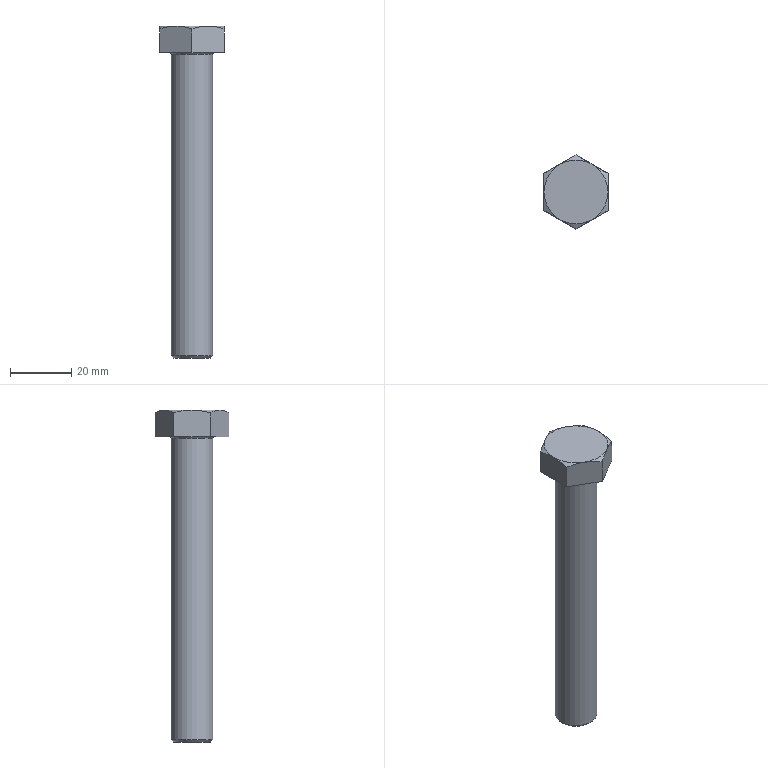Part | NX | 1 solid | 18 faces | box 21 x 24.249 x 108.8 mm | volume 18047 mm3 | plane 9 | cone 7 | cylinder 1 | torus 1 | commonest cylinder face diameters 13.682 x1
STEP:
#1=CARTESIAN_POINT('',(7.441,0.,0.));
#2=VERTEX_POINT('',#1);
#3=CARTESIAN_POINT('',(0.,0.,0.));
#4=DIRECTION('',(0.,0.,1.));
#5=DIRECTION('',(1.,0.,0.));
#6=AXIS2_PLACEMENT_3D('',#3,#4,#5);
#7=CIRCLE('',#6,7.441);
#8=EDGE_CURVE('',#2,#2,#7,.T.);
#9=ORIENTED_EDGE('',*,*,#8,.T.);
#10=EDGE_LOOP('',(#9));
#11=FACE_BOUND('',#10,.T.);
#12=CARTESIAN_POINT('',(0.,12.124,0.));
#13=VERTEX_POINT('',#12);
#14=CARTESIAN_POINT('',(10.5,6.062,0.));
#15=VERTEX_POINT('',#14);
#16=CARTESIAN_POINT('',(0.,12.124,0.));
#17=DIRECTION('',(0.866,-0.5,0.));
#18=VECTOR('',#17,1.);
#19=LINE('',#16,#18);
#20=EDGE_CURVE('',#13,#15,#19,.T.);
#21=ORIENTED_EDGE('',*,*,#20,.T.);
#22=CARTESIAN_POINT('',(10.5,-6.062,0.));
#23=VERTEX_POINT('',#22);
#24=CARTESIAN_POINT('',(10.5,6.062,0.));
#25=DIRECTION('',(0.,-1.,0.));
#26=VECTOR('',#25,1.);
#27=LINE('',#24,#26);
#28=EDGE_CURVE('',#15,#23,#27,.T.);
#29=ORIENTED_EDGE('',*,*,#28,.T.);
#30=CARTESIAN_POINT('',(0.,-12.124,0.));
#31=VERTEX_POINT('',#30);
#32=CARTESIAN_POINT('',(10.5,-6.062,0.));
#33=DIRECTION('',(-0.866,-0.5,0.));
#34=VECTOR('',#33,1.);
#35=LINE('',#32,#34);
#36=EDGE_CURVE('',#23,#31,#35,.T.);
#37=ORIENTED_EDGE('',*,*,#36,.T.);
#38=CARTESIAN_POINT('',(-10.5,-6.062,0.));
#39=VERTEX_POINT('',#38);
#40=CARTESIAN_POINT('',(0.,-12.124,0.));
#41=DIRECTION('',(-0.866,0.5,0.));
#42=VECTOR('',#41,1.);
#43=LINE('',#40,#42);
#44=EDGE_CURVE('',#31,#39,#43,.T.);
#45=ORIENTED_EDGE('',*,*,#44,.T.);
#46=CARTESIAN_POINT('',(-10.5,6.062,0.));
#47=VERTEX_POINT('',#46);
#48=CARTESIAN_POINT('',(-10.5,-6.062,0.));
#49=DIRECTION('',(0.,1.,0.));
#50=VECTOR('',#49,1.);
#51=LINE('',#48,#50);
#52=EDGE_CURVE('',#39,#47,#51,.T.);
#53=ORIENTED_EDGE('',*,*,#52,.T.);
#54=CARTESIAN_POINT('',(-10.5,6.062,0.));
#55=DIRECTION('',(0.866,0.5,0.));
#56=VECTOR('',#55,1.);
#57=LINE('',#54,#56);
#58=EDGE_CURVE('',#47,#13,#57,.T.);
#59=ORIENTED_EDGE('',*,*,#58,.T.);
#60=EDGE_LOOP('',(#21,#29,#37,#45,#53,#59));
#61=FACE_BOUND('',#60,.T.);
#62=CARTESIAN_POINT('',(-10.5,18.187,0.));
#63=DIRECTION('',(0.,0.,1.));
#64=DIRECTION('',(-1.,0.,0.));
#65=AXIS2_PLACEMENT_3D('',#62,#63,#64);
#66=PLANE('',#65);
#67=ADVANCED_FACE('',(#11,#61),#66,.F.);
#68=CARTESIAN_POINT('',(10.5,6.062,7.862));
#69=VERTEX_POINT('',#68);
#70=CARTESIAN_POINT('',(5.25,9.093,8.8));
#71=VERTEX_POINT('',#70);
#72=CARTESIAN_POINT('',(10.5,6.062,7.862));
#73=CARTESIAN_POINT('',(8.785,7.052,8.434));
#74=CARTESIAN_POINT('',(7.042,8.059,8.8));
#75=CARTESIAN_POINT('',(5.25,9.093,8.8));
#76=B_SPLINE_CURVE_WITH_KNOTS('',3,(#72,#73,#74,#75),.UNSPECIFIED.,.F.,.F.,(4,4),(0.,1.),.UNSPECIFIED.);
#77=EDGE_CURVE('',#69,#71,#76,.T.);
#78=ORIENTED_EDGE('',*,*,#77,.F.);
#79=CARTESIAN_POINT('',(10.5,6.062,8.8));
#80=DIRECTION('',(0.,0.,-1.));
#81=VECTOR('',#80,1.);
#82=LINE('',#79,#81);
#83=EDGE_CURVE('',#69,#15,#82,.T.);
#84=ORIENTED_EDGE('',*,*,#83,.T.);
#85=ORIENTED_EDGE('',*,*,#20,.F.);
#86=CARTESIAN_POINT('',(0.,12.124,7.862));
#87=VERTEX_POINT('',#86);
#88=CARTESIAN_POINT('',(0.,12.124,8.8));
#89=DIRECTION('',(0.,0.,-1.));
#90=VECTOR('',#89,1.);
#91=LINE('',#88,#90);
#92=EDGE_CURVE('',#87,#13,#91,.T.);
#93=ORIENTED_EDGE('',*,*,#92,.F.);
#94=CARTESIAN_POINT('',(5.25,9.093,8.8));
#95=CARTESIAN_POINT('',(3.458,10.128,8.8));
#96=CARTESIAN_POINT('',(1.715,11.134,8.434));
#97=CARTESIAN_POINT('',(0.,12.124,7.862));
#98=B_SPLINE_CURVE_WITH_KNOTS('',3,(#94,#95,#96,#97),.UNSPECIFIED.,.F.,.F.,(4,4),(0.,1.),.UNSPECIFIED.);
#99=EDGE_CURVE('',#71,#87,#98,.T.);
#100=ORIENTED_EDGE('',*,*,#99,.F.);
#101=EDGE_LOOP('',(#78,#84,#85,#93,#100));
#102=FACE_OUTER_BOUND('',#101,.T.);
#103=CARTESIAN_POINT('',(0.,12.124,8.8));
#104=DIRECTION('',(0.5,0.866,0.));
#105=DIRECTION('',(0.866,-0.5,0.));
#106=AXIS2_PLACEMENT_3D('',#103,#104,#105);
#107=PLANE('',#106);
#108=ADVANCED_FACE('',(#102),#107,.T.);
#109=CARTESIAN_POINT('',(10.5,-6.062,7.862));
#110=VERTEX_POINT('',#109);
#111=CARTESIAN_POINT('',(10.5,0.,8.8));
#112=VERTEX_POINT('',#111);
#113=CARTESIAN_POINT('',(10.5,-6.062,7.862));
#114=CARTESIAN_POINT('',(10.5,-4.082,8.434));
#115=CARTESIAN_POINT('',(10.5,-2.069,8.8));
#116=CARTESIAN_POINT('',(10.5,0.,8.8));
#117=B_SPLINE_CURVE_WITH_KNOTS('',3,(#113,#114,#115,#116),.UNSPECIFIED.,.F.,.F.,(4,4),(0.,1.),.UNSPECIFIED.);
#118=EDGE_CURVE('',#110,#112,#117,.T.);
#119=ORIENTED_EDGE('',*,*,#118,.F.);
#120=CARTESIAN_POINT('',(10.5,-6.062,8.8));
#121=DIRECTION('',(0.,0.,-1.));
#122=VECTOR('',#121,1.);
#123=LINE('',#120,#122);
#124=EDGE_CURVE('',#110,#23,#123,.T.);
#125=ORIENTED_EDGE('',*,*,#124,.T.);
#126=ORIENTED_EDGE('',*,*,#28,.F.);
#127=ORIENTED_EDGE('',*,*,#83,.F.);
#128=CARTESIAN_POINT('',(10.5,0.,8.8));
#129=CARTESIAN_POINT('',(10.5,2.069,8.8));
#130=CARTESIAN_POINT('',(10.5,4.082,8.434));
#131=CARTESIAN_POINT('',(10.5,6.062,7.862));
#132=B_SPLINE_CURVE_WITH_KNOTS('',3,(#128,#129,#130,#131),.UNSPECIFIED.,.F.,.F.,(4,4),(0.,1.),.UNSPECIFIED.);
#133=EDGE_CURVE('',#112,#69,#132,.T.);
#134=ORIENTED_EDGE('',*,*,#133,.F.);
#135=EDGE_LOOP('',(#119,#125,#126,#127,#134));
#136=FACE_OUTER_BOUND('',#135,.T.);
#137=CARTESIAN_POINT('',(10.5,6.062,8.8));
#138=DIRECTION('',(1.,0.,0.));
#139=DIRECTION('',(0.,-1.,0.));
#140=AXIS2_PLACEMENT_3D('',#137,#138,#139);
#141=PLANE('',#140);
#142=ADVANCED_FACE('',(#136),#141,.T.);
#143=CARTESIAN_POINT('',(0.,-12.124,7.862));
#144=VERTEX_POINT('',#143);
#145=CARTESIAN_POINT('',(5.25,-9.093,8.8));
#146=VERTEX_POINT('',#145);
#147=CARTESIAN_POINT('',(0.,-12.124,7.862));
#148=CARTESIAN_POINT('',(1.715,-11.134,8.434));
#149=CARTESIAN_POINT('',(3.458,-10.128,8.8));
#150=CARTESIAN_POINT('',(5.25,-9.093,8.8));
#151=B_SPLINE_CURVE_WITH_KNOTS('',3,(#147,#148,#149,#150),.UNSPECIFIED.,.F.,.F.,(4,4),(0.,1.),.UNSPECIFIED.);
#152=EDGE_CURVE('',#144,#146,#151,.T.);
#153=ORIENTED_EDGE('',*,*,#152,.F.);
#154=CARTESIAN_POINT('',(0.,-12.124,8.8));
#155=DIRECTION('',(0.,0.,-1.));
#156=VECTOR('',#155,1.);
#157=LINE('',#154,#156);
#158=EDGE_CURVE('',#144,#31,#157,.T.);
#159=ORIENTED_EDGE('',*,*,#158,.T.);
#160=ORIENTED_EDGE('',*,*,#36,.F.);
#161=ORIENTED_EDGE('',*,*,#124,.F.);
#162=CARTESIAN_POINT('',(5.25,-9.093,8.8));
#163=CARTESIAN_POINT('',(7.042,-8.059,8.8));
#164=CARTESIAN_POINT('',(8.785,-7.052,8.434));
#165=CARTESIAN_POINT('',(10.5,-6.062,7.862));
#166=B_SPLINE_CURVE_WITH_KNOTS('',3,(#162,#163,#164,#165),.UNSPECIFIED.,.F.,.F.,(4,4),(0.,1.),.UNSPECIFIED.);
#167=EDGE_CURVE('',#146,#110,#166,.T.);
#168=ORIENTED_EDGE('',*,*,#167,.F.);
#169=EDGE_LOOP('',(#153,#159,#160,#161,#168));
#170=FACE_OUTER_BOUND('',#169,.T.);
#171=CARTESIAN_POINT('',(10.5,-6.062,8.8));
#172=DIRECTION('',(0.5,-0.866,0.));
#173=DIRECTION('',(-0.866,-0.5,0.));
#174=AXIS2_PLACEMENT_3D('',#171,#172,#173);
#175=PLANE('',#174);
#176=ADVANCED_FACE('',(#170),#175,.T.);
#177=CARTESIAN_POINT('',(-10.5,-6.062,7.862));
#178=VERTEX_POINT('',#177);
#179=CARTESIAN_POINT('',(-5.25,-9.093,8.8));
#180=VERTEX_POINT('',#179);
#181=CARTESIAN_POINT('',(-10.5,-6.062,7.862));
#182=CARTESIAN_POINT('',(-8.785,-7.052,8.434));
#183=CARTESIAN_POINT('',(-7.042,-8.059,8.8));
#184=CARTESIAN_POINT('',(-5.25,-9.093,8.8));
#185=B_SPLINE_CURVE_WITH_KNOTS('',3,(#181,#182,#183,#184),.UNSPECIFIED.,.F.,.F.,(4,4),(0.,1.),.UNSPECIFIED.);
#186=EDGE_CURVE('',#178,#180,#185,.T.);
#187=ORIENTED_EDGE('',*,*,#186,.F.);
#188=CARTESIAN_POINT('',(-10.5,-6.062,8.8));
#189=DIRECTION('',(0.,0.,-1.));
#190=VECTOR('',#189,1.);
#191=LINE('',#188,#190);
#192=EDGE_CURVE('',#178,#39,#191,.T.);
#193=ORIENTED_EDGE('',*,*,#192,.T.);
#194=ORIENTED_EDGE('',*,*,#44,.F.);
#195=ORIENTED_EDGE('',*,*,#158,.F.);
#196=CARTESIAN_POINT('',(-5.25,-9.093,8.8));
#197=CARTESIAN_POINT('',(-3.458,-10.128,8.8));
#198=CARTESIAN_POINT('',(-1.715,-11.134,8.434));
#199=CARTESIAN_POINT('',(0.,-12.124,7.862));
#200=B_SPLINE_CURVE_WITH_KNOTS('',3,(#196,#197,#198,#199),.UNSPECIFIED.,.F.,.F.,(4,4),(0.,1.),.UNSPECIFIED.);
#201=EDGE_CURVE('',#180,#144,#200,.T.);
#202=ORIENTED_EDGE('',*,*,#201,.F.);
#203=EDGE_LOOP('',(#187,#193,#194,#195,#202));
#204=FACE_OUTER_BOUND('',#203,.T.);
#205=CARTESIAN_POINT('',(0.,-12.124,8.8));
#206=DIRECTION('',(-0.5,-0.866,0.));
#207=DIRECTION('',(-0.866,0.5,0.));
#208=AXIS2_PLACEMENT_3D('',#205,#206,#207);
#209=PLANE('',#208);
#210=ADVANCED_FACE('',(#204),#209,.T.);
#211=CARTESIAN_POINT('',(-10.5,6.062,7.862));
#212=VERTEX_POINT('',#211);
#213=CARTESIAN_POINT('',(-10.5,0.,8.8));
#214=VERTEX_POINT('',#213);
#215=CARTESIAN_POINT('',(-10.5,6.062,7.862));
#216=CARTESIAN_POINT('',(-10.5,4.082,8.434));
#217=CARTESIAN_POINT('',(-10.5,2.069,8.8));
#218=CARTESIAN_POINT('',(-10.5,0.,8.8));
#219=B_SPLINE_CURVE_WITH_KNOTS('',3,(#215,#216,#217,#218),.UNSPECIFIED.,.F.,.F.,(4,4),(0.,1.),.UNSPECIFIED.);
#220=EDGE_CURVE('',#212,#214,#219,.T.);
#221=ORIENTED_EDGE('',*,*,#220,.F.);
#222=CARTESIAN_POINT('',(-10.5,6.062,8.8));
#223=DIRECTION('',(0.,0.,-1.));
#224=VECTOR('',#223,1.);
#225=LINE('',#222,#224);
#226=EDGE_CURVE('',#212,#47,#225,.T.);
#227=ORIENTED_EDGE('',*,*,#226,.T.);
#228=ORIENTED_EDGE('',*,*,#52,.F.);
#229=ORIENTED_EDGE('',*,*,#192,.F.);
#230=CARTESIAN_POINT('',(-10.5,0.,8.8));
#231=CARTESIAN_POINT('',(-10.5,-2.069,8.8));
#232=CARTESIAN_POINT('',(-10.5,-4.082,8.434));
#233=CARTESIAN_POINT('',(-10.5,-6.062,7.862));
#234=B_SPLINE_CURVE_WITH_KNOTS('',3,(#230,#231,#232,#233),.UNSPECIFIED.,.F.,.F.,(4,4),(0.,1.),.UNSPECIFIED.);
#235=EDGE_CURVE('',#214,#178,#234,.T.);
#236=ORIENTED_EDGE('',*,*,#235,.F.);
#237=EDGE_LOOP('',(#221,#227,#228,#229,#236));
#238=FACE_OUTER_BOUND('',#237,.T.);
#239=CARTESIAN_POINT('',(-10.5,-6.062,8.8));
#240=DIRECTION('',(-1.,0.,0.));
#241=DIRECTION('',(0.,0.,-1.));
#242=AXIS2_PLACEMENT_3D('',#239,#240,#241);
#243=PLANE('',#242);
#244=ADVANCED_FACE('',(#238),#243,.T.);
#245=CARTESIAN_POINT('',(-5.25,9.093,8.8));
#246=VERTEX_POINT('',#245);
#247=CARTESIAN_POINT('',(0.,12.124,7.862));
#248=CARTESIAN_POINT('',(-1.715,11.134,8.434));
#249=CARTESIAN_POINT('',(-3.458,10.128,8.8));
#250=CARTESIAN_POINT('',(-5.25,9.093,8.8));
#251=B_SPLINE_CURVE_WITH_KNOTS('',3,(#247,#248,#249,#250),.UNSPECIFIED.,.F.,.F.,(4,4),(0.,1.),.UNSPECIFIED.);
#252=EDGE_CURVE('',#87,#246,#251,.T.);
#253=ORIENTED_EDGE('',*,*,#252,.F.);
#254=ORIENTED_EDGE('',*,*,#92,.T.);
#255=ORIENTED_EDGE('',*,*,#58,.F.);
#256=ORIENTED_EDGE('',*,*,#226,.F.);
#257=CARTESIAN_POINT('',(-5.25,9.093,8.8));
#258=CARTESIAN_POINT('',(-7.042,8.059,8.8));
#259=CARTESIAN_POINT('',(-8.785,7.052,8.434));
#260=CARTESIAN_POINT('',(-10.5,6.062,7.862));
#261=B_SPLINE_CURVE_WITH_KNOTS('',3,(#257,#258,#259,#260),.UNSPECIFIED.,.F.,.F.,(4,4),(0.,1.),.UNSPECIFIED.);
#262=EDGE_CURVE('',#246,#212,#261,.T.);
#263=ORIENTED_EDGE('',*,*,#262,.F.);
#264=EDGE_LOOP('',(#253,#254,#255,#256,#263));
#265=FACE_OUTER_BOUND('',#264,.T.);
#266=CARTESIAN_POINT('',(-10.5,6.062,8.8));
#267=DIRECTION('',(-0.5,0.866,0.));
#268=DIRECTION('',(0.866,0.5,0.));
#269=AXIS2_PLACEMENT_3D('',#266,#267,#268);
#270=PLANE('',#269);
#271=ADVANCED_FACE('',(#265),#270,.T.);
#272=CARTESIAN_POINT('',(-6.841,0.,-99.316));
#273=VERTEX_POINT('',#272);
#274=CARTESIAN_POINT('',(0.,0.,-99.316));
#275=DIRECTION('',(0.,0.,1.));
#276=DIRECTION('',(-1.,0.,0.));
#277=AXIS2_PLACEMENT_3D('',#274,#275,#276);
#278=CIRCLE('',#277,6.841);
#279=EDGE_CURVE('',#273,#273,#278,.T.);
#280=ORIENTED_EDGE('',*,*,#279,.T.);
#281=EDGE_LOOP('',(#280));
#282=FACE_BOUND('',#281,.T.);
#283=CARTESIAN_POINT('',(6.841,0.,-0.6));
#284=VERTEX_POINT('',#283);
#285=CARTESIAN_POINT('',(0.,0.,-0.6));
#286=DIRECTION('',(0.,0.,-1.));
#287=DIRECTION('',(1.,0.,0.));
#288=AXIS2_PLACEMENT_3D('',#285,#286,#287);
#289=CIRCLE('',#288,6.841);
#290=EDGE_CURVE('',#284,#284,#289,.T.);
#291=ORIENTED_EDGE('',*,*,#290,.T.);
#292=EDGE_LOOP('',(#291));
#293=FACE_BOUND('',#292,.T.);
#294=CARTESIAN_POINT('',(0.,0.,-100.));
#295=DIRECTION('',(0.,0.,1.));
#296=DIRECTION('',(-1.,0.,0.));
#297=AXIS2_PLACEMENT_3D('',#294,#295,#296);
#298=CYLINDRICAL_SURFACE('',#297,6.841);
#299=ADVANCED_FACE('',(#282,#293),#298,.T.);
#300=CARTESIAN_POINT('',(-6.157,0.,-100.));
#301=VERTEX_POINT('',#300);
#302=CARTESIAN_POINT('',(0.,0.,-100.));
#303=DIRECTION('',(0.,0.,-1.));
#304=DIRECTION('',(-1.,0.,0.));
#305=AXIS2_PLACEMENT_3D('',#302,#303,#304);
#306=CIRCLE('',#305,6.157);
#307=EDGE_CURVE('',#301,#301,#306,.T.);
#308=ORIENTED_EDGE('',*,*,#307,.T.);
#309=EDGE_LOOP('',(#308));
#310=FACE_OUTER_BOUND('',#309,.T.);
#311=CARTESIAN_POINT('',(0.,0.,-100.));
#312=DIRECTION('',(0.,0.,-1.));
#313=DIRECTION('',(1.,0.,0.));
#314=AXIS2_PLACEMENT_3D('',#311,#312,#313);
#315=PLANE('',#314);
#316=ADVANCED_FACE('',(#310),#315,.T.);
#317=ORIENTED_EDGE('',*,*,#220,.T.);
#318=CARTESIAN_POINT('',(0.,0.,8.8));
#319=DIRECTION('',(0.,0.,-1.));
#320=DIRECTION('',(-1.,0.,0.));
#321=AXIS2_PLACEMENT_3D('',#318,#319,#320);
#322=CIRCLE('',#321,10.5);
#323=EDGE_CURVE('',#214,#246,#322,.T.);
#324=ORIENTED_EDGE('',*,*,#323,.T.);
#325=ORIENTED_EDGE('',*,*,#262,.T.);
#326=EDGE_LOOP('',(#317,#324,#325));
#327=FACE_OUTER_BOUND('',#326,.T.);
#328=CARTESIAN_POINT('',(0.,0.,8.8));
#329=DIRECTION('',(0.,0.,-1.));
#330=DIRECTION('',(1.,0.,0.));
#331=AXIS2_PLACEMENT_3D('',#328,#329,#330);
#332=CONICAL_SURFACE('',#331,10.5,60.);
#333=ADVANCED_FACE('',(#327),#332,.T.);
#334=ORIENTED_EDGE('',*,*,#99,.T.);
#335=ORIENTED_EDGE('',*,*,#252,.T.);
#336=CARTESIAN_POINT('',(0.,0.,8.8));
#337=DIRECTION('',(0.,0.,-1.));
#338=DIRECTION('',(-1.,0.,0.));
#339=AXIS2_PLACEMENT_3D('',#336,#337,#338);
#340=CIRCLE('',#339,10.5);
#341=EDGE_CURVE('',#246,#71,#340,.T.);
#342=ORIENTED_EDGE('',*,*,#341,.T.);
#343=EDGE_LOOP('',(#334,#335,#342));
#344=FACE_OUTER_BOUND('',#343,.T.);
#345=CARTESIAN_POINT('',(0.,0.,8.8));
#346=DIRECTION('',(0.,0.,-1.));
#347=DIRECTION('',(1.,0.,0.));
#348=AXIS2_PLACEMENT_3D('',#345,#346,#347);
#349=CONICAL_SURFACE('',#348,10.5,60.);
#350=ADVANCED_FACE('',(#344),#349,.T.);
#351=ORIENTED_EDGE('',*,*,#186,.T.);
#352=CARTESIAN_POINT('',(0.,0.,8.8));
#353=DIRECTION('',(0.,0.,-1.));
#354=DIRECTION('',(-1.,0.,0.));
#355=AXIS2_PLACEMENT_3D('',#352,#353,#354);
#356=CIRCLE('',#355,10.5);
#357=EDGE_CURVE('',#180,#214,#356,.T.);
#358=ORIENTED_EDGE('',*,*,#357,.T.);
#359=ORIENTED_EDGE('',*,*,#235,.T.);
#360=EDGE_LOOP('',(#351,#358,#359));
#361=FACE_OUTER_BOUND('',#360,.T.);
#362=CARTESIAN_POINT('',(0.,0.,8.8));
#363=DIRECTION('',(0.,0.,-1.));
#364=DIRECTION('',(1.,0.,0.));
#365=AXIS2_PLACEMENT_3D('',#362,#363,#364);
#366=CONICAL_SURFACE('',#365,10.5,60.);
#367=ADVANCED_FACE('',(#361),#366,.T.);
#368=ORIENTED_EDGE('',*,*,#152,.T.);
#369=CARTESIAN_POINT('',(0.,0.,8.8));
#370=DIRECTION('',(0.,0.,-1.));
#371=DIRECTION('',(-1.,0.,0.));
#372=AXIS2_PLACEMENT_3D('',#369,#370,#371);
#373=CIRCLE('',#372,10.5);
#374=EDGE_CURVE('',#146,#180,#373,.T.);
#375=ORIENTED_EDGE('',*,*,#374,.T.);
#376=ORIENTED_EDGE('',*,*,#201,.T.);
#377=EDGE_LOOP('',(#368,#375,#376));
#378=FACE_OUTER_BOUND('',#377,.T.);
#379=CARTESIAN_POINT('',(0.,0.,8.8));
#380=DIRECTION('',(0.,0.,-1.));
#381=DIRECTION('',(1.,0.,0.));
#382=AXIS2_PLACEMENT_3D('',#379,#380,#381);
#383=CONICAL_SURFACE('',#382,10.5,60.);
#384=ADVANCED_FACE('',(#378),#383,.T.);
#385=ORIENTED_EDGE('',*,*,#167,.T.);
#386=ORIENTED_EDGE('',*,*,#118,.T.);
#387=CARTESIAN_POINT('',(0.,0.,8.8));
#388=DIRECTION('',(0.,0.,-1.));
#389=DIRECTION('',(-1.,0.,0.));
#390=AXIS2_PLACEMENT_3D('',#387,#388,#389);
#391=CIRCLE('',#390,10.5);
#392=EDGE_CURVE('',#112,#146,#391,.T.);
#393=ORIENTED_EDGE('',*,*,#392,.T.);
#394=EDGE_LOOP('',(#385,#386,#393));
#395=FACE_OUTER_BOUND('',#394,.T.);
#396=CARTESIAN_POINT('',(0.,0.,8.8));
#397=DIRECTION('',(0.,0.,-1.));
#398=DIRECTION('',(1.,0.,0.));
#399=AXIS2_PLACEMENT_3D('',#396,#397,#398);
#400=CONICAL_SURFACE('',#399,10.5,60.);
#401=ADVANCED_FACE('',(#395),#400,.T.);
#402=ORIENTED_EDGE('',*,*,#133,.T.);
#403=ORIENTED_EDGE('',*,*,#77,.T.);
#404=CARTESIAN_POINT('',(0.,0.,8.8));
#405=DIRECTION('',(0.,0.,-1.));
#406=DIRECTION('',(-1.,0.,0.));
#407=AXIS2_PLACEMENT_3D('',#404,#405,#406);
#408=CIRCLE('',#407,10.5);
#409=EDGE_CURVE('',#71,#112,#408,.T.);
#410=ORIENTED_EDGE('',*,*,#409,.T.);
#411=EDGE_LOOP('',(#402,#403,#410));
#412=FACE_OUTER_BOUND('',#411,.T.);
#413=CARTESIAN_POINT('',(0.,0.,8.8));
#414=DIRECTION('',(0.,0.,-1.));
#415=DIRECTION('',(1.,0.,0.));
#416=AXIS2_PLACEMENT_3D('',#413,#414,#415);
#417=CONICAL_SURFACE('',#416,10.5,60.);
#418=ADVANCED_FACE('',(#412),#417,.T.);
#419=ORIENTED_EDGE('',*,*,#323,.F.);
#420=ORIENTED_EDGE('',*,*,#357,.F.);
#421=ORIENTED_EDGE('',*,*,#374,.F.);
#422=ORIENTED_EDGE('',*,*,#392,.F.);
#423=ORIENTED_EDGE('',*,*,#409,.F.);
#424=ORIENTED_EDGE('',*,*,#341,.F.);
#425=EDGE_LOOP('',(#419,#420,#421,#422,#423,#424));
#426=FACE_OUTER_BOUND('',#425,.T.);
#427=CARTESIAN_POINT('',(-10.5,18.187,8.8));
#428=DIRECTION('',(0.,0.,1.));
#429=DIRECTION('',(-1.,0.,0.));
#430=AXIS2_PLACEMENT_3D('',#427,#428,#429);
#431=PLANE('',#430);
#432=ADVANCED_FACE('',(#426),#431,.T.);
#433=ORIENTED_EDGE('',*,*,#8,.F.);
#434=EDGE_LOOP('',(#433));
#435=FACE_BOUND('',#434,.T.);
#436=ORIENTED_EDGE('',*,*,#290,.F.);
#437=EDGE_LOOP('',(#436));
#438=FACE_BOUND('',#437,.T.);
#439=CARTESIAN_POINT('',(0.,0.,-0.6));
#440=DIRECTION('',(0.,0.,1.));
#441=DIRECTION('',(-1.,0.,0.));
#442=AXIS2_PLACEMENT_3D('',#439,#440,#441);
#443=TOROIDAL_SURFACE('',#442,7.441,0.6);
#444=ADVANCED_FACE('',(#435,#438),#443,.F.);
#445=ORIENTED_EDGE('',*,*,#279,.F.);
#446=EDGE_LOOP('',(#445));
#447=FACE_BOUND('',#446,.T.);
#448=ORIENTED_EDGE('',*,*,#307,.F.);
#449=EDGE_LOOP('',(#448));
#450=FACE_BOUND('',#449,.T.);
#451=CARTESIAN_POINT('',(0.,0.,-100.));
#452=DIRECTION('',(0.,0.,1.));
#453=DIRECTION('',(-1.,0.,0.));
#454=AXIS2_PLACEMENT_3D('',#451,#452,#453);
#455=CONICAL_SURFACE('',#454,6.157,45.);
#456=ADVANCED_FACE('',(#447,#450),#455,.T.);
#457=CLOSED_SHELL('',(#67,#108,#142,#176,#210,#244,#271,#299,#316,#333,#350,#367,#384,#401,#418,#432,#444,#456));
#458=MANIFOLD_SOLID_BREP('',#457);
#459=(LENGTH_UNIT()NAMED_UNIT(*)SI_UNIT(.MILLI.,.METRE.));
#460=UNCERTAINTY_MEASURE_WITH_UNIT(LENGTH_MEASURE(0.0508),#459,'','');
#461=(NAMED_UNIT(*)PLANE_ANGLE_UNIT()SI_UNIT($,.RADIAN.));
#462=PLANE_ANGLE_MEASURE_WITH_UNIT(PLANE_ANGLE_MEASURE(0.01745),#461);
#463=DIMENSIONAL_EXPONENTS(0.,0.,0.,0.,0.,0.,0.);
#464=(CONVERSION_BASED_UNIT('DEGREE',#462)NAMED_UNIT(#463)PLANE_ANGLE_UNIT());
#465=(NAMED_UNIT(*)SI_UNIT($,.STERADIAN.)SOLID_ANGLE_UNIT());
#466=(GEOMETRIC_REPRESENTATION_CONTEXT(3)GLOBAL_UNCERTAINTY_ASSIGNED_CONTEXT((#460))GLOBAL_UNIT_ASSIGNED_CONTEXT((#459,#464,#465))REPRESENTATION_CONTEXT('',''));
#467=ADVANCED_BREP_SHAPE_REPRESENTATION('',(#458),#466);